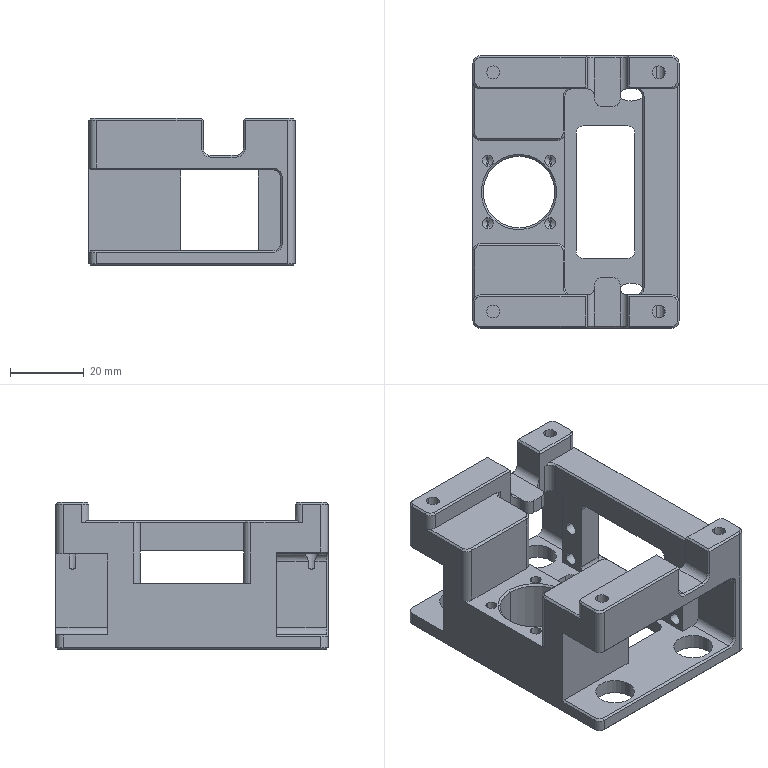Part | 1 solid | 236 faces | box 56 x 74 x 40 mm | volume 53076 mm3 | plane 102 | cylinder 80 | cone 54 | commonest cylinder face diameters 4 x46 3.5 x16 3 x8 10.5 x8 19.5 x2